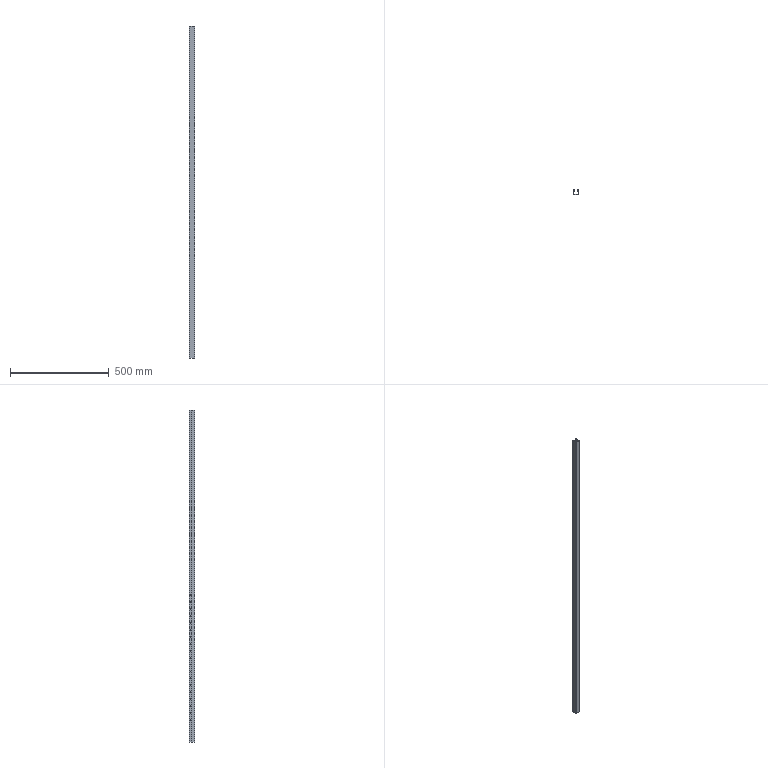Part | STEP file | GALVANIZED RAIL 023 | 1 solid | 120 faces | box 28.4 x 26.2 x 1678 mm | volume 167389 mm3 | cylinder 92 | plane 28 | commonest cylinder face diameters 4 x76 1.473 x8 3.873 x8